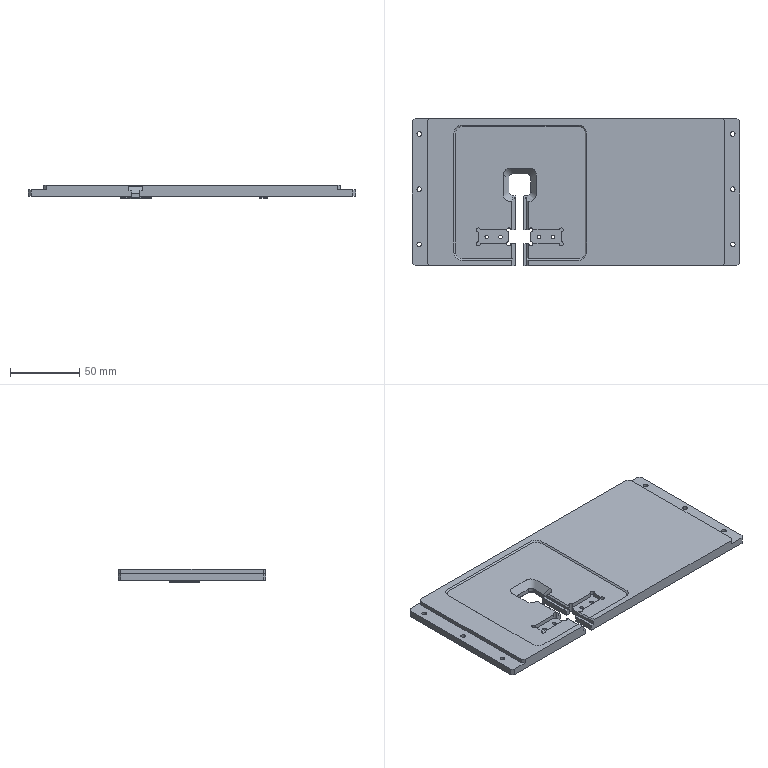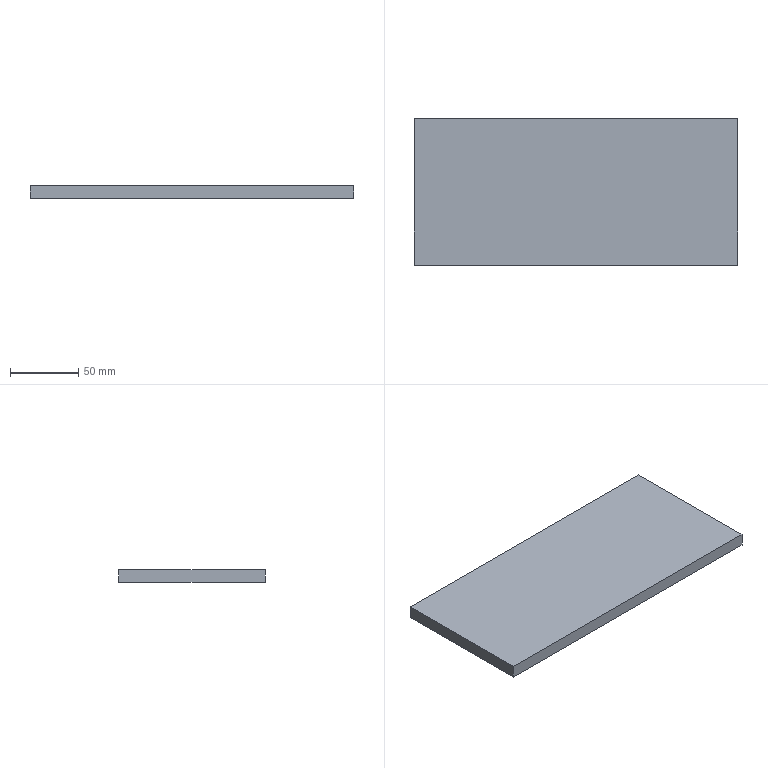CAM job | NX | 3-axis milling, drilling | part box 237 x 107 x 9.5 mm | stock box 237 x 107 x 9.5 mm
Tools:
number,name,description,diameter,corner_radius,flute_length,length,flutes
20,D10,Milling Tool-5 Parameters,10.0,0.0,50.0,75.0,2
11,D10JING,Milling Tool-5 Parameters,10.0,0.0,50.0,75.0,2
22,D6A45,Milling Tool-5 Parameters,6.0,0.0,3.0,3.0,2
1,ZXZ,Milling Tool-5 Parameters,6.0,0.0,50.0,75.0,2
19,3.3ZT,Drilling Tool,3.3,0.0,35.0,50.0,2
21,2.5ZT,Drilling Tool,2.4,0.0,35.0,50.0,2
24,3.0ZT,Drilling Tool,3.0,0.0,35.0,50.0,2
6,D6,Milling Tool-5 Parameters,6.0,0.0,50.0,75.0,2
7,D6JING,Milling Tool-5 Parameters,6.0,0.0,50.0,75.0,2
4,D4,Milling Tool-5 Parameters,4.0,0.0,50.0,75.0,2
5,D4JING,Milling Tool-5 Parameters,4.0,0.0,50.0,75.0,2
23,D6R0.5,Milling Tool-5 Parameters,6.0,0.5,50.0,75.0,2
Operations:
program,operation,operation_type,tool,method,geometry_group,spindle_rpm,surface_speed,feed_per_tooth,feed_cut,feed_plunge,cut_length_mm,path_length_mm,cut_time_min,machine_time_min
1吸,DRILLING_COPY_1_COPY_1,Operation,ZXZ,METHOD,A,5000.0,94.0,0.025,250.0,0.0,72.0,694.981,0.288,0.3503
1吸,DRILLING_COPY_1_COPY_COPY_COPY_COPY_1_COPY,Operation,3.3ZT,METHOD,A,2000.0,20.0,0.0375,120.0,0.0,73.8,610.069,0.615,0.6686
1吸,DRILLING_COPY_1_COPY_COPY_COPY_COPY_1_COPY_COPY,Operation,2.5ZT,METHOD,A,2000.0,20.0,0.0375,100.0,0.0,49.2,216.441,0.492,0.5087
1吸,DRILLING_COPY_1_COPY_COPY_COPY_COPY_1_COPY_COPY_1,Operation,3.0ZT,METHOD,A,2000.0,20.0,0.0375,120.0,0.0,31.605,213.166,0.2634,0.2815
1吸,DRILLING_COPY_1_COPY_COPY_COPY_COPY_1_COPY_COPY_1_COPY,Operation,3.0ZT,METHOD,A,2000.0,20.0,0.0375,120.0,0.0,49.2,204.559,0.41,0.4255
1吸,CAVITY_MILL,CavityMilling,D10,METHOD,A,2800.0,87.0,0.3929,2200.0,1000.0,19991.626,27887.614,10.281,11.071
1吸,ZLEVEL_PROFILE_COPY_COPY_COPY_COPY_1_COPY,ZLevelMilling,D6,METHOD,A,3500.0,65.0,0.2,1400.0,100.0,1397.592,1469.942,0.9983,1.006
1吸,CAVITY_MILL_COPY,CavityMilling,D6,METHOD,A,3800.0,71.0,0.2171,1650.0,1000.0,10968.006,14146.355,7.313,7.631
1吸,CAVITY_MILL_COPY_COPY,CavityMilling,D4,METHOD,A,4500.0,56.0,0.1833,1650.0,1000.0,7226.562,9001.474,4.896,5.074
1吸,FLOOR_WALL_1_1,VolumeBased25DMillingOperation,D6JING,METHOD,A,7000.0,219.0,0.0714,1000.0,100.0,4971.125,7188.27,4.971,5.193
1吸,ZLEVEL_PROFILE_1_COPY,ZLevelMilling,D4JING,METHOD,A,7500.0,141.0,0.0833,1250.0,100.0,169.339,243.339,0.1355,0.1429
1吸,ZLEVEL_PROFILE_1_COPY_COPY,ZLevelMilling,D4JING,METHOD,A,7500.0,141.0,0.0833,1250.0,100.0,51.214,127.914,0.041,0.0486
1吸,ZLEVEL_PROFILE_1_COPY_COPY_1,ZLevelMilling,D6R0.5,METHOD,A,7500.0,141.0,0.1467,2200.0,100.0,5238.582,5297.653,2.381,2.387
1吸,ZLEVEL_PROFILE_1_COPY_COPY_1_COPY,ZLevelMilling,D6R0.5,METHOD,A,7500.0,141.0,0.1467,2200.0,100.0,5091.035,5224.594,2.314,2.328
1吸,ZLEVEL_PROFILE_1_COPY_COPY_1_COPY_COPY,ZLevelMilling,D6R0.5,METHOD,A,7500.0,141.0,0.1467,2200.0,100.0,1528.996,1837.086,0.695,0.7258
1吸,ZLEVEL_PROFILE_1_COPY_COPY_1_COPY_COPY_COPY,ZLevelMilling,D6R0.5,METHOD,A,7500.0,141.0,0.1467,2200.0,100.0,326.948,455.193,0.1486,0.1614
1吸,ZLEVEL_PROFILE_1_COPY_1_COPY,ZLevelMilling,D6A45,METHOD,A,7500.0,141.0,0.0667,1000.0,100.0,636.97,696.97,0.637,0.643
1吸,ZLEVEL_PROFILE_1_COPY_1_COPY_COPY,ZLevelMilling,D6A45,METHOD,A,7500.0,141.0,0.0667,1000.0,100.0,311.195,2061.606,0.3112,0.4862
2,CAVITY_MILL_COPY_1,CavityMilling,D10,METHOD,B,2800.0,87.0,0.3929,2200.0,1000.0,29644.687,30401.675,13.503,13.579
2,CAVITY_MILL_COPY_1_COPY,CavityMilling,D10,METHOD,B,2800.0,87.0,0.3929,2200.0,1000.0,6474.12,7341.918,3.373,3.46
2,CAVITY_MILL_COPY_COPY_1,CavityMilling,D6,METHOD,B,3800.0,71.0,0.2171,1650.0,1000.0,2035.928,5273.685,1.461,1.785
2,FLOOR_WALL_1_1_COPY,VolumeBased25DMillingOperation,D10JING,METHOD,B,7000.0,219.0,0.0714,1000.0,100.0,6148.636,6769.487,6.149,6.211
2,ZLEVEL_PROFILE_1_COPY_COPY_1_COPY_1,ZLevelMilling,D6R0.5,METHOD,B,7500.0,141.0,0.1467,2200.0,100.0,5058.56,5494.698,2.299,2.343
2,ZLEVEL_PROFILE_1_COPY_1_COPY_COPY_1,ZLevelMilling,D6A45,METHOD,B,7500.0,141.0,0.0667,1000.0,100.0,1058.704,3009.999,1.059,1.254